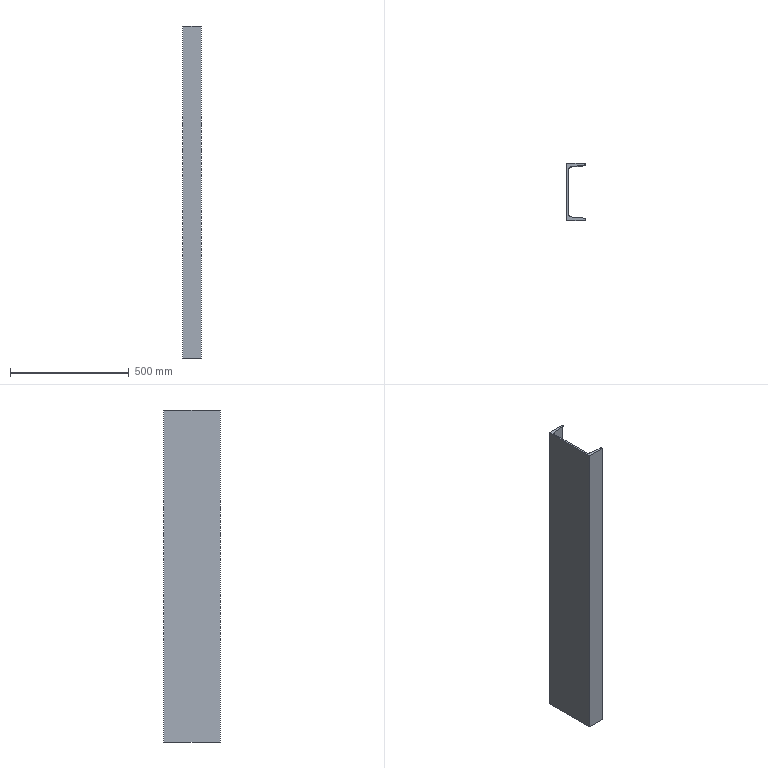Part | NX | features BREP 1 | 1 solid | 14 faces | box 78 x 240 x 1400 mm | volume 4711916 mm3 | plane 10 | cylinder 4 | commonest cylinder face diameters 12 x2 24 x2
STEP:
#1=CARTESIAN_POINT('',(72.,110.95,-700.));
#2=VERTEX_POINT('',#1);
#3=CARTESIAN_POINT('',(78.,116.95,-700.));
#4=VERTEX_POINT('',#3);
#5=CARTESIAN_POINT('',(72.,116.95,-700.));
#6=DIRECTION('',(0.,0.,1.));
#7=DIRECTION('',(-1.,0.,0.));
#8=AXIS2_PLACEMENT_3D('',#5,#6,#7);
#9=CIRCLE('',#8,6.);
#10=EDGE_CURVE('',#2,#4,#9,.T.);
#11=ORIENTED_EDGE('',*,*,#10,.T.);
#12=CARTESIAN_POINT('',(78.,116.95,700.));
#13=VERTEX_POINT('',#12);
#14=CARTESIAN_POINT('',(78.,116.95,700.));
#15=DIRECTION('',(0.,0.,-1.));
#16=VECTOR('',#15,1000.);
#17=LINE('',#14,#16);
#18=EDGE_CURVE('',#13,#4,#17,.T.);
#19=ORIENTED_EDGE('',*,*,#18,.F.);
#20=CARTESIAN_POINT('',(72.,110.95,700.));
#21=VERTEX_POINT('',#20);
#22=CARTESIAN_POINT('',(72.,116.95,700.));
#23=DIRECTION('',(0.,0.,1.));
#24=DIRECTION('',(-1.,0.,0.));
#25=AXIS2_PLACEMENT_3D('',#22,#23,#24);
#26=CIRCLE('',#25,6.);
#27=EDGE_CURVE('',#21,#13,#26,.T.);
#28=ORIENTED_EDGE('',*,*,#27,.F.);
#29=CARTESIAN_POINT('',(72.,110.95,700.));
#30=DIRECTION('',(0.,0.,-1.));
#31=VECTOR('',#30,1000.);
#32=LINE('',#29,#31);
#33=EDGE_CURVE('',#21,#2,#32,.T.);
#34=ORIENTED_EDGE('',*,*,#33,.T.);
#35=EDGE_LOOP('',(#11,#19,#28,#34));
#36=FACE_BOUND('',#35,.T.);
#37=CARTESIAN_POINT('',(72.,116.95,700.));
#38=DIRECTION('',(0.,0.,-1.));
#39=DIRECTION('',(1.,0.,0.));
#40=AXIS2_PLACEMENT_3D('',#37,#38,#39);
#41=CYLINDRICAL_SURFACE('',#40,6.);
#42=ADVANCED_FACE('',(#36),#41,.T.);
#43=CARTESIAN_POINT('',(78.,120.,-700.));
#44=VERTEX_POINT('',#43);
#45=CARTESIAN_POINT('',(78.,120.,-700.));
#46=DIRECTION('',(0.,1.,0.));
#47=VECTOR('',#46,1000.);
#48=LINE('',#45,#47);
#49=EDGE_CURVE('',#4,#44,#48,.T.);
#50=ORIENTED_EDGE('',*,*,#49,.T.);
#51=CARTESIAN_POINT('',(78.,120.,700.));
#52=VERTEX_POINT('',#51);
#53=CARTESIAN_POINT('',(78.,120.,700.));
#54=DIRECTION('',(0.,0.,-1.));
#55=VECTOR('',#54,1000.);
#56=LINE('',#53,#55);
#57=EDGE_CURVE('',#52,#44,#56,.T.);
#58=ORIENTED_EDGE('',*,*,#57,.F.);
#59=CARTESIAN_POINT('',(78.,120.,700.));
#60=DIRECTION('',(0.,1.,0.));
#61=VECTOR('',#60,1000.);
#62=LINE('',#59,#61);
#63=EDGE_CURVE('',#13,#52,#62,.T.);
#64=ORIENTED_EDGE('',*,*,#63,.F.);
#65=ORIENTED_EDGE('',*,*,#18,.T.);
#66=EDGE_LOOP('',(#50,#58,#64,#65));
#67=FACE_BOUND('',#66,.T.);
#68=CARTESIAN_POINT('',(78.,120.,700.));
#69=DIRECTION('',(-1.,0.,0.));
#70=DIRECTION('',(0.,0.,-1.));
#71=AXIS2_PLACEMENT_3D('',#68,#69,#70);
#72=PLANE('',#71);
#73=ADVANCED_FACE('',(#67),#72,.F.);
#74=CARTESIAN_POINT('',(0.,120.,-700.));
#75=VERTEX_POINT('',#74);
#76=CARTESIAN_POINT('',(0.,120.,-700.));
#77=DIRECTION('',(-1.,0.,0.));
#78=VECTOR('',#77,1000.);
#79=LINE('',#76,#78);
#80=EDGE_CURVE('',#44,#75,#79,.T.);
#81=ORIENTED_EDGE('',*,*,#80,.T.);
#82=CARTESIAN_POINT('',(0.,120.,700.));
#83=VERTEX_POINT('',#82);
#84=CARTESIAN_POINT('',(0.,120.,700.));
#85=DIRECTION('',(0.,0.,-1.));
#86=VECTOR('',#85,1000.);
#87=LINE('',#84,#86);
#88=EDGE_CURVE('',#83,#75,#87,.T.);
#89=ORIENTED_EDGE('',*,*,#88,.F.);
#90=CARTESIAN_POINT('',(0.,120.,700.));
#91=DIRECTION('',(-1.,0.,0.));
#92=VECTOR('',#91,1000.);
#93=LINE('',#90,#92);
#94=EDGE_CURVE('',#52,#83,#93,.T.);
#95=ORIENTED_EDGE('',*,*,#94,.F.);
#96=ORIENTED_EDGE('',*,*,#57,.T.);
#97=EDGE_LOOP('',(#81,#89,#95,#96));
#98=FACE_BOUND('',#97,.T.);
#99=CARTESIAN_POINT('',(0.,120.,700.));
#100=DIRECTION('',(0.,-1.,0.));
#101=DIRECTION('',(0.,0.,1.));
#102=AXIS2_PLACEMENT_3D('',#99,#100,#101);
#103=PLANE('',#102);
#104=ADVANCED_FACE('',(#98),#103,.F.);
#105=CARTESIAN_POINT('',(0.,-120.,-700.));
#106=VERTEX_POINT('',#105);
#107=CARTESIAN_POINT('',(0.,120.,-700.));
#108=DIRECTION('',(0.,-1.,0.));
#109=VECTOR('',#108,1000.);
#110=LINE('',#107,#109);
#111=EDGE_CURVE('',#75,#106,#110,.T.);
#112=ORIENTED_EDGE('',*,*,#111,.T.);
#113=CARTESIAN_POINT('',(0.,-120.,700.));
#114=VERTEX_POINT('',#113);
#115=CARTESIAN_POINT('',(0.,-120.,700.));
#116=DIRECTION('',(0.,0.,-1.));
#117=VECTOR('',#116,1000.);
#118=LINE('',#115,#117);
#119=EDGE_CURVE('',#114,#106,#118,.T.);
#120=ORIENTED_EDGE('',*,*,#119,.F.);
#121=CARTESIAN_POINT('',(0.,120.,700.));
#122=DIRECTION('',(0.,-1.,0.));
#123=VECTOR('',#122,1000.);
#124=LINE('',#121,#123);
#125=EDGE_CURVE('',#83,#114,#124,.T.);
#126=ORIENTED_EDGE('',*,*,#125,.F.);
#127=ORIENTED_EDGE('',*,*,#88,.T.);
#128=EDGE_LOOP('',(#112,#120,#126,#127));
#129=FACE_BOUND('',#128,.T.);
#130=CARTESIAN_POINT('',(0.,120.,700.));
#131=DIRECTION('',(1.,0.,0.));
#132=DIRECTION('',(0.,0.,1.));
#133=AXIS2_PLACEMENT_3D('',#130,#131,#132);
#134=PLANE('',#133);
#135=ADVANCED_FACE('',(#129),#134,.F.);
#136=CARTESIAN_POINT('',(78.,-120.,-700.));
#137=VERTEX_POINT('',#136);
#138=CARTESIAN_POINT('',(0.,-120.,-700.));
#139=DIRECTION('',(1.,0.,0.));
#140=VECTOR('',#139,1000.);
#141=LINE('',#138,#140);
#142=EDGE_CURVE('',#106,#137,#141,.T.);
#143=ORIENTED_EDGE('',*,*,#142,.T.);
#144=CARTESIAN_POINT('',(78.,-120.,700.));
#145=VERTEX_POINT('',#144);
#146=CARTESIAN_POINT('',(78.,-120.,700.));
#147=DIRECTION('',(0.,0.,-1.));
#148=VECTOR('',#147,1000.);
#149=LINE('',#146,#148);
#150=EDGE_CURVE('',#145,#137,#149,.T.);
#151=ORIENTED_EDGE('',*,*,#150,.F.);
#152=CARTESIAN_POINT('',(0.,-120.,700.));
#153=DIRECTION('',(1.,0.,0.));
#154=VECTOR('',#153,1000.);
#155=LINE('',#152,#154);
#156=EDGE_CURVE('',#114,#145,#155,.T.);
#157=ORIENTED_EDGE('',*,*,#156,.F.);
#158=ORIENTED_EDGE('',*,*,#119,.T.);
#159=EDGE_LOOP('',(#143,#151,#157,#158));
#160=FACE_BOUND('',#159,.T.);
#161=CARTESIAN_POINT('',(0.,-120.,700.));
#162=DIRECTION('',(0.,1.,0.));
#163=DIRECTION('',(0.,0.,-1.));
#164=AXIS2_PLACEMENT_3D('',#161,#162,#163);
#165=PLANE('',#164);
#166=ADVANCED_FACE('',(#160),#165,.F.);
#167=CARTESIAN_POINT('',(78.,-116.95,-700.));
#168=VERTEX_POINT('',#167);
#169=CARTESIAN_POINT('',(78.,-120.,-700.));
#170=DIRECTION('',(0.,1.,0.));
#171=VECTOR('',#170,1000.);
#172=LINE('',#169,#171);
#173=EDGE_CURVE('',#137,#168,#172,.T.);
#174=ORIENTED_EDGE('',*,*,#173,.T.);
#175=CARTESIAN_POINT('',(78.,-116.95,700.));
#176=VERTEX_POINT('',#175);
#177=CARTESIAN_POINT('',(78.,-116.95,700.));
#178=DIRECTION('',(0.,0.,-1.));
#179=VECTOR('',#178,1000.);
#180=LINE('',#177,#179);
#181=EDGE_CURVE('',#176,#168,#180,.T.);
#182=ORIENTED_EDGE('',*,*,#181,.F.);
#183=CARTESIAN_POINT('',(78.,-120.,700.));
#184=DIRECTION('',(0.,1.,0.));
#185=VECTOR('',#184,1000.);
#186=LINE('',#183,#185);
#187=EDGE_CURVE('',#145,#176,#186,.T.);
#188=ORIENTED_EDGE('',*,*,#187,.F.);
#189=ORIENTED_EDGE('',*,*,#150,.T.);
#190=EDGE_LOOP('',(#174,#182,#188,#189));
#191=FACE_BOUND('',#190,.T.);
#192=CARTESIAN_POINT('',(78.,-120.,700.));
#193=DIRECTION('',(-1.,0.,0.));
#194=DIRECTION('',(0.,0.,-1.));
#195=AXIS2_PLACEMENT_3D('',#192,#193,#194);
#196=PLANE('',#195);
#197=ADVANCED_FACE('',(#191),#196,.F.);
#198=CARTESIAN_POINT('',(72.,-110.95,-700.));
#199=VERTEX_POINT('',#198);
#200=CARTESIAN_POINT('',(72.,-116.95,-700.));
#201=DIRECTION('',(0.,0.,1.));
#202=DIRECTION('',(1.,0.,0.));
#203=AXIS2_PLACEMENT_3D('',#200,#201,#202);
#204=CIRCLE('',#203,6.);
#205=EDGE_CURVE('',#168,#199,#204,.T.);
#206=ORIENTED_EDGE('',*,*,#205,.T.);
#207=CARTESIAN_POINT('',(72.,-110.95,700.));
#208=VERTEX_POINT('',#207);
#209=CARTESIAN_POINT('',(72.,-110.95,700.));
#210=DIRECTION('',(0.,0.,-1.));
#211=VECTOR('',#210,1000.);
#212=LINE('',#209,#211);
#213=EDGE_CURVE('',#208,#199,#212,.T.);
#214=ORIENTED_EDGE('',*,*,#213,.F.);
#215=CARTESIAN_POINT('',(72.,-116.95,700.));
#216=DIRECTION('',(0.,0.,1.));
#217=DIRECTION('',(1.,0.,0.));
#218=AXIS2_PLACEMENT_3D('',#215,#216,#217);
#219=CIRCLE('',#218,6.);
#220=EDGE_CURVE('',#176,#208,#219,.T.);
#221=ORIENTED_EDGE('',*,*,#220,.F.);
#222=ORIENTED_EDGE('',*,*,#181,.T.);
#223=EDGE_LOOP('',(#206,#214,#221,#222));
#224=FACE_BOUND('',#223,.T.);
#225=CARTESIAN_POINT('',(72.,-116.95,700.));
#226=DIRECTION('',(0.,0.,-1.));
#227=DIRECTION('',(1.,0.,0.));
#228=AXIS2_PLACEMENT_3D('',#225,#226,#227);
#229=CYLINDRICAL_SURFACE('',#228,6.);
#230=ADVANCED_FACE('',(#224),#229,.T.);
#231=CARTESIAN_POINT('',(19.,-106.35,-700.));
#232=VERTEX_POINT('',#231);
#233=CARTESIAN_POINT('',(72.,-110.95,-700.));
#234=DIRECTION('',(-0.9963,0.08647,0.));
#235=VECTOR('',#234,1000.);
#236=LINE('',#233,#235);
#237=EDGE_CURVE('',#199,#232,#236,.T.);
#238=ORIENTED_EDGE('',*,*,#237,.T.);
#239=CARTESIAN_POINT('',(19.,-106.35,700.));
#240=VERTEX_POINT('',#239);
#241=CARTESIAN_POINT('',(19.,-106.35,700.));
#242=DIRECTION('',(0.,0.,-1.));
#243=VECTOR('',#242,1000.);
#244=LINE('',#241,#243);
#245=EDGE_CURVE('',#240,#232,#244,.T.);
#246=ORIENTED_EDGE('',*,*,#245,.F.);
#247=CARTESIAN_POINT('',(72.,-110.95,700.));
#248=DIRECTION('',(-0.9963,0.08647,0.));
#249=VECTOR('',#248,1000.);
#250=LINE('',#247,#249);
#251=EDGE_CURVE('',#208,#240,#250,.T.);
#252=ORIENTED_EDGE('',*,*,#251,.F.);
#253=ORIENTED_EDGE('',*,*,#213,.T.);
#254=EDGE_LOOP('',(#238,#246,#252,#253));
#255=FACE_BOUND('',#254,.T.);
#256=CARTESIAN_POINT('',(72.,-110.95,700.));
#257=DIRECTION('',(-0.08647,-0.9963,0.));
#258=DIRECTION('',(-0.9963,0.08647,0.));
#259=AXIS2_PLACEMENT_3D('',#256,#257,#258);
#260=PLANE('',#259);
#261=ADVANCED_FACE('',(#255),#260,.F.);
#262=CARTESIAN_POINT('',(7.,-94.35,-700.));
#263=VERTEX_POINT('',#262);
#264=CARTESIAN_POINT('',(19.,-94.35,-700.));
#265=DIRECTION('',(0.,0.,-1.));
#266=DIRECTION('',(1.,0.,0.));
#267=AXIS2_PLACEMENT_3D('',#264,#265,#266);
#268=CIRCLE('',#267,12.);
#269=EDGE_CURVE('',#232,#263,#268,.T.);
#270=ORIENTED_EDGE('',*,*,#269,.T.);
#271=CARTESIAN_POINT('',(7.,-94.35,700.));
#272=VERTEX_POINT('',#271);
#273=CARTESIAN_POINT('',(7.,-94.35,700.));
#274=DIRECTION('',(0.,0.,-1.));
#275=VECTOR('',#274,1000.);
#276=LINE('',#273,#275);
#277=EDGE_CURVE('',#272,#263,#276,.T.);
#278=ORIENTED_EDGE('',*,*,#277,.F.);
#279=CARTESIAN_POINT('',(19.,-94.35,700.));
#280=DIRECTION('',(0.,0.,-1.));
#281=DIRECTION('',(1.,0.,0.));
#282=AXIS2_PLACEMENT_3D('',#279,#280,#281);
#283=CIRCLE('',#282,12.);
#284=EDGE_CURVE('',#240,#272,#283,.T.);
#285=ORIENTED_EDGE('',*,*,#284,.F.);
#286=ORIENTED_EDGE('',*,*,#245,.T.);
#287=EDGE_LOOP('',(#270,#278,#285,#286));
#288=FACE_BOUND('',#287,.T.);
#289=CARTESIAN_POINT('',(19.,-94.35,700.));
#290=DIRECTION('',(0.,0.,-1.));
#291=DIRECTION('',(1.,0.,0.));
#292=AXIS2_PLACEMENT_3D('',#289,#290,#291);
#293=CYLINDRICAL_SURFACE('',#292,12.);
#294=ADVANCED_FACE('',(#288),#293,.F.);
#295=CARTESIAN_POINT('',(7.,94.35,-700.));
#296=VERTEX_POINT('',#295);
#297=CARTESIAN_POINT('',(7.,-94.35,-700.));
#298=DIRECTION('',(0.,1.,0.));
#299=VECTOR('',#298,1000.);
#300=LINE('',#297,#299);
#301=EDGE_CURVE('',#263,#296,#300,.T.);
#302=ORIENTED_EDGE('',*,*,#301,.T.);
#303=CARTESIAN_POINT('',(7.,94.35,700.));
#304=VERTEX_POINT('',#303);
#305=CARTESIAN_POINT('',(7.,94.35,700.));
#306=DIRECTION('',(0.,0.,-1.));
#307=VECTOR('',#306,1000.);
#308=LINE('',#305,#307);
#309=EDGE_CURVE('',#304,#296,#308,.T.);
#310=ORIENTED_EDGE('',*,*,#309,.F.);
#311=CARTESIAN_POINT('',(7.,-94.35,700.));
#312=DIRECTION('',(0.,1.,0.));
#313=VECTOR('',#312,1000.);
#314=LINE('',#311,#313);
#315=EDGE_CURVE('',#272,#304,#314,.T.);
#316=ORIENTED_EDGE('',*,*,#315,.F.);
#317=ORIENTED_EDGE('',*,*,#277,.T.);
#318=EDGE_LOOP('',(#302,#310,#316,#317));
#319=FACE_BOUND('',#318,.T.);
#320=CARTESIAN_POINT('',(7.,-94.35,700.));
#321=DIRECTION('',(-1.,0.,0.));
#322=DIRECTION('',(0.,0.,-1.));
#323=AXIS2_PLACEMENT_3D('',#320,#321,#322);
#324=PLANE('',#323);
#325=ADVANCED_FACE('',(#319),#324,.F.);
#326=CARTESIAN_POINT('',(19.,106.35,-700.));
#327=VERTEX_POINT('',#326);
#328=CARTESIAN_POINT('',(19.,94.35,-700.));
#329=DIRECTION('',(0.,0.,-1.));
#330=DIRECTION('',(-1.,0.,0.));
#331=AXIS2_PLACEMENT_3D('',#328,#329,#330);
#332=CIRCLE('',#331,12.);
#333=EDGE_CURVE('',#296,#327,#332,.T.);
#334=ORIENTED_EDGE('',*,*,#333,.T.);
#335=CARTESIAN_POINT('',(19.,106.35,700.));
#336=VERTEX_POINT('',#335);
#337=CARTESIAN_POINT('',(19.,106.35,700.));
#338=DIRECTION('',(0.,0.,-1.));
#339=VECTOR('',#338,1000.);
#340=LINE('',#337,#339);
#341=EDGE_CURVE('',#336,#327,#340,.T.);
#342=ORIENTED_EDGE('',*,*,#341,.F.);
#343=CARTESIAN_POINT('',(19.,94.35,700.));
#344=DIRECTION('',(0.,0.,-1.));
#345=DIRECTION('',(-1.,0.,0.));
#346=AXIS2_PLACEMENT_3D('',#343,#344,#345);
#347=CIRCLE('',#346,12.);
#348=EDGE_CURVE('',#304,#336,#347,.T.);
#349=ORIENTED_EDGE('',*,*,#348,.F.);
#350=ORIENTED_EDGE('',*,*,#309,.T.);
#351=EDGE_LOOP('',(#334,#342,#349,#350));
#352=FACE_BOUND('',#351,.T.);
#353=CARTESIAN_POINT('',(19.,94.35,700.));
#354=DIRECTION('',(0.,0.,-1.));
#355=DIRECTION('',(1.,0.,0.));
#356=AXIS2_PLACEMENT_3D('',#353,#354,#355);
#357=CYLINDRICAL_SURFACE('',#356,12.);
#358=ADVANCED_FACE('',(#352),#357,.F.);
#359=CARTESIAN_POINT('',(72.,110.95,-700.));
#360=DIRECTION('',(0.9963,0.08647,0.));
#361=VECTOR('',#360,1000.);
#362=LINE('',#359,#361);
#363=EDGE_CURVE('',#327,#2,#362,.T.);
#364=ORIENTED_EDGE('',*,*,#363,.T.);
#365=ORIENTED_EDGE('',*,*,#33,.F.);
#366=CARTESIAN_POINT('',(72.,110.95,700.));
#367=DIRECTION('',(0.9963,0.08647,0.));
#368=VECTOR('',#367,1000.);
#369=LINE('',#366,#368);
#370=EDGE_CURVE('',#336,#21,#369,.T.);
#371=ORIENTED_EDGE('',*,*,#370,.F.);
#372=ORIENTED_EDGE('',*,*,#341,.T.);
#373=EDGE_LOOP('',(#364,#365,#371,#372));
#374=FACE_BOUND('',#373,.T.);
#375=CARTESIAN_POINT('',(72.,110.95,700.));
#376=DIRECTION('',(-0.08647,0.9963,0.));
#377=DIRECTION('',(0.9963,0.08647,0.));
#378=AXIS2_PLACEMENT_3D('',#375,#376,#377);
#379=PLANE('',#378);
#380=ADVANCED_FACE('',(#374),#379,.F.);
#381=ORIENTED_EDGE('',*,*,#27,.T.);
#382=ORIENTED_EDGE('',*,*,#63,.T.);
#383=ORIENTED_EDGE('',*,*,#94,.T.);
#384=ORIENTED_EDGE('',*,*,#125,.T.);
#385=ORIENTED_EDGE('',*,*,#156,.T.);
#386=ORIENTED_EDGE('',*,*,#187,.T.);
#387=ORIENTED_EDGE('',*,*,#220,.T.);
#388=ORIENTED_EDGE('',*,*,#251,.T.);
#389=ORIENTED_EDGE('',*,*,#284,.T.);
#390=ORIENTED_EDGE('',*,*,#315,.T.);
#391=ORIENTED_EDGE('',*,*,#348,.T.);
#392=ORIENTED_EDGE('',*,*,#370,.T.);
#393=EDGE_LOOP('',(#381,#382,#383,#384,#385,#386,#387,#388,#389,#390,#391,#392));
#394=FACE_BOUND('',#393,.T.);
#395=CARTESIAN_POINT('',(72.,116.95,700.));
#396=DIRECTION('',(0.,0.,-1.));
#397=DIRECTION('',(1.,0.,0.));
#398=AXIS2_PLACEMENT_3D('',#395,#396,#397);
#399=PLANE('',#398);
#400=ADVANCED_FACE('',(#394),#399,.F.);
#401=ORIENTED_EDGE('',*,*,#10,.F.);
#402=ORIENTED_EDGE('',*,*,#363,.F.);
#403=ORIENTED_EDGE('',*,*,#333,.F.);
#404=ORIENTED_EDGE('',*,*,#301,.F.);
#405=ORIENTED_EDGE('',*,*,#269,.F.);
#406=ORIENTED_EDGE('',*,*,#237,.F.);
#407=ORIENTED_EDGE('',*,*,#205,.F.);
#408=ORIENTED_EDGE('',*,*,#173,.F.);
#409=ORIENTED_EDGE('',*,*,#142,.F.);
#410=ORIENTED_EDGE('',*,*,#111,.F.);
#411=ORIENTED_EDGE('',*,*,#80,.F.);
#412=ORIENTED_EDGE('',*,*,#49,.F.);
#413=EDGE_LOOP('',(#401,#402,#403,#404,#405,#406,#407,#408,#409,#410,#411,#412));
#414=FACE_BOUND('',#413,.T.);
#415=CARTESIAN_POINT('',(72.,116.95,-700.));
#416=DIRECTION('',(0.,0.,-1.));
#417=DIRECTION('',(1.,0.,0.));
#418=AXIS2_PLACEMENT_3D('',#415,#416,#417);
#419=PLANE('',#418);
#420=ADVANCED_FACE('',(#414),#419,.T.);
#421=CLOSED_SHELL('',(#42,#73,#104,#135,#166,#197,#230,#261,#294,#325,#358,#380,#400,#420));
#422=MANIFOLD_SOLID_BREP('',#421);
#423=(LENGTH_UNIT()NAMED_UNIT(*)SI_UNIT(.MILLI.,.METRE.));
#424=UNCERTAINTY_MEASURE_WITH_UNIT(LENGTH_MEASURE(0.00001),#423,'','');
#425=(NAMED_UNIT(*)PLANE_ANGLE_UNIT()SI_UNIT($,.RADIAN.));
#426=(NAMED_UNIT(*)SI_UNIT($,.STERADIAN.)SOLID_ANGLE_UNIT());
#427=(GEOMETRIC_REPRESENTATION_CONTEXT(3)GLOBAL_UNCERTAINTY_ASSIGNED_CONTEXT((#424))GLOBAL_UNIT_ASSIGNED_CONTEXT((#423,#425,#426))REPRESENTATION_CONTEXT('',''));
#428=ADVANCED_BREP_SHAPE_REPRESENTATION('',(#422),#427);